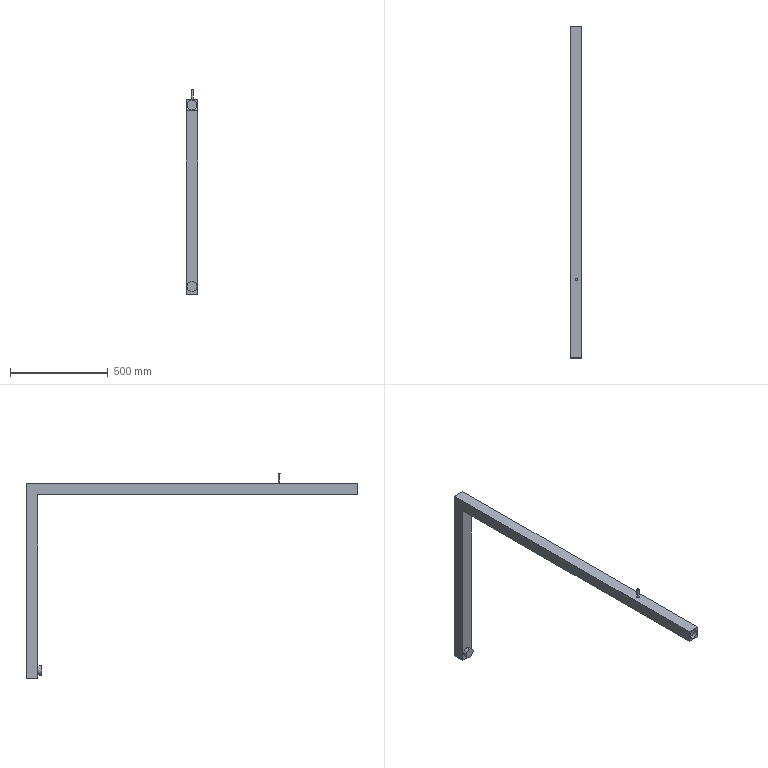Part | SolidWorks | features BaseBody 1 | 1 solid | 17 faces | box 60 x 1700 x 1049 mm | volume 9509525 mm3 | plane 11 | cylinder 6 | commonest cylinder face diameters 50 x4 12 x2
STEP:
#1=CARTESIAN_POINT('',(0.,1699.2,-991.929));
#2=VERTEX_POINT('',#1);
#3=CARTESIAN_POINT('',(0.,1699.2,-1041.929));
#4=VERTEX_POINT('',#3);
#5=CARTESIAN_POINT('',(0.,1699.2,-1016.929));
#6=DIRECTION('',(0.,1.,0.));
#7=DIRECTION('',(0.,0.,1.));
#8=AXIS2_PLACEMENT_3D('',#5,#6,#7);
#9=CIRCLE('',#8,25.);
#10=EDGE_CURVE('',#2,#4,#9,.T.);
#11=ORIENTED_EDGE('',*,*,#10,.T.);
#12=CARTESIAN_POINT('',(0.,1719.2,-1041.929));
#13=VERTEX_POINT('',#12);
#14=CARTESIAN_POINT('',(0.,1699.2,-1041.929));
#15=DIRECTION('',(0.,1.,0.));
#16=VECTOR('',#15,1000.);
#17=LINE('',#14,#16);
#18=EDGE_CURVE('',#4,#13,#17,.T.);
#19=ORIENTED_EDGE('',*,*,#18,.T.);
#20=CARTESIAN_POINT('',(0.,1719.2,-991.929));
#21=VERTEX_POINT('',#20);
#22=CARTESIAN_POINT('',(0.,1719.2,-1016.929));
#23=DIRECTION('',(0.,-1.,0.));
#24=DIRECTION('',(0.,0.,1.));
#25=AXIS2_PLACEMENT_3D('',#22,#23,#24);
#26=CIRCLE('',#25,25.);
#27=EDGE_CURVE('',#13,#21,#26,.T.);
#28=ORIENTED_EDGE('',*,*,#27,.T.);
#29=CARTESIAN_POINT('',(0.,1699.2,-991.929));
#30=DIRECTION('',(0.,1.,0.));
#31=VECTOR('',#30,1000.);
#32=LINE('',#29,#31);
#33=EDGE_CURVE('',#2,#21,#32,.T.);
#34=ORIENTED_EDGE('',*,*,#33,.F.);
#35=EDGE_LOOP('',(#11,#19,#28,#34));
#36=FACE_OUTER_BOUND('',#35,.T.);
#37=CARTESIAN_POINT('',(0.,1699.2,-1016.929));
#38=DIRECTION('',(0.,1.,0.));
#39=DIRECTION('',(0.,0.,1.));
#40=AXIS2_PLACEMENT_3D('',#37,#38,#39);
#41=CYLINDRICAL_SURFACE('',#40,25.);
#42=ADVANCED_FACE('',(#36),#41,.T.);
#43=CARTESIAN_POINT('',(0.,99.2,-62.879));
#44=VERTEX_POINT('',#43);
#45=CARTESIAN_POINT('',(0.,99.2,-112.879));
#46=VERTEX_POINT('',#45);
#47=CARTESIAN_POINT('',(0.,99.2,-87.879));
#48=DIRECTION('',(0.,-1.,0.));
#49=DIRECTION('',(0.,0.,-1.));
#50=AXIS2_PLACEMENT_3D('',#47,#48,#49);
#51=CIRCLE('',#50,25.);
#52=EDGE_CURVE('',#44,#46,#51,.T.);
#53=ORIENTED_EDGE('',*,*,#52,.F.);
#54=CARTESIAN_POINT('',(0.,79.2,-62.879));
#55=VERTEX_POINT('',#54);
#56=CARTESIAN_POINT('',(0.,99.2,-62.879));
#57=DIRECTION('',(0.,-1.,0.));
#58=VECTOR('',#57,1000.);
#59=LINE('',#56,#58);
#60=EDGE_CURVE('',#44,#55,#59,.T.);
#61=ORIENTED_EDGE('',*,*,#60,.T.);
#62=CARTESIAN_POINT('',(0.,79.2,-112.879));
#63=VERTEX_POINT('',#62);
#64=CARTESIAN_POINT('',(0.,79.2,-87.879));
#65=DIRECTION('',(0.,-1.,0.));
#66=DIRECTION('',(0.,0.,-1.));
#67=AXIS2_PLACEMENT_3D('',#64,#65,#66);
#68=CIRCLE('',#67,25.);
#69=EDGE_CURVE('',#55,#63,#68,.T.);
#70=ORIENTED_EDGE('',*,*,#69,.T.);
#71=CARTESIAN_POINT('',(0.,99.2,-112.879));
#72=DIRECTION('',(0.,-1.,0.));
#73=VECTOR('',#72,1000.);
#74=LINE('',#71,#73);
#75=EDGE_CURVE('',#46,#63,#74,.T.);
#76=ORIENTED_EDGE('',*,*,#75,.F.);
#77=EDGE_LOOP('',(#53,#61,#70,#76));
#78=FACE_OUTER_BOUND('',#77,.T.);
#79=CARTESIAN_POINT('',(0.,99.2,-87.879));
#80=DIRECTION('',(0.,-1.,0.));
#81=DIRECTION('',(0.,0.,-1.));
#82=AXIS2_PLACEMENT_3D('',#79,#80,#81);
#83=CYLINDRICAL_SURFACE('',#82,25.);
#84=ADVANCED_FACE('',(#78),#83,.F.);
#85=CARTESIAN_POINT('',(-4.497,482.123,-9.029));
#86=VERTEX_POINT('',#85);
#87=CARTESIAN_POINT('',(7.503,482.123,-9.029));
#88=VERTEX_POINT('',#87);
#89=CARTESIAN_POINT('',(1.503,482.123,-9.029));
#90=DIRECTION('',(0.,0.,-1.));
#91=DIRECTION('',(-1.,0.,0.));
#92=AXIS2_PLACEMENT_3D('',#89,#90,#91);
#93=CIRCLE('',#92,6.);
#94=EDGE_CURVE('',#86,#88,#93,.T.);
#95=ORIENTED_EDGE('',*,*,#94,.T.);
#96=CARTESIAN_POINT('',(7.503,482.123,-57.879));
#97=VERTEX_POINT('',#96);
#98=CARTESIAN_POINT('',(7.503,482.123,7.942));
#99=DIRECTION('',(0.,0.,-1.));
#100=VECTOR('',#99,1000.);
#101=LINE('',#98,#100);
#102=EDGE_CURVE('',#88,#97,#101,.T.);
#103=ORIENTED_EDGE('',*,*,#102,.T.);
#104=CARTESIAN_POINT('',(-4.497,482.123,-57.879));
#105=VERTEX_POINT('',#104);
#106=CARTESIAN_POINT('',(1.503,482.123,-57.879));
#107=DIRECTION('',(0.,0.,1.));
#108=DIRECTION('',(-1.,0.,0.));
#109=AXIS2_PLACEMENT_3D('',#106,#107,#108);
#110=CIRCLE('',#109,6.);
#111=EDGE_CURVE('',#97,#105,#110,.T.);
#112=ORIENTED_EDGE('',*,*,#111,.T.);
#113=CARTESIAN_POINT('',(-4.497,482.123,7.942));
#114=DIRECTION('',(0.,0.,-1.));
#115=VECTOR('',#114,1000.);
#116=LINE('',#113,#115);
#117=EDGE_CURVE('',#86,#105,#116,.T.);
#118=ORIENTED_EDGE('',*,*,#117,.F.);
#119=EDGE_LOOP('',(#95,#103,#112,#118));
#120=FACE_OUTER_BOUND('',#119,.T.);
#121=CARTESIAN_POINT('',(1.503,482.123,7.942));
#122=DIRECTION('',(0.,0.,-1.));
#123=DIRECTION('',(-1.,0.,0.));
#124=AXIS2_PLACEMENT_3D('',#121,#122,#123);
#125=CYLINDRICAL_SURFACE('',#124,6.);
#126=ADVANCED_FACE('',(#120),#125,.T.);
#127=CARTESIAN_POINT('',(30.,1719.2,-1057.879));
#128=VERTEX_POINT('',#127);
#129=CARTESIAN_POINT('',(30.,1779.2,-1057.879));
#130=VERTEX_POINT('',#129);
#131=CARTESIAN_POINT('',(30.,1133.527,-1057.879));
#132=DIRECTION('',(0.,1.,0.));
#133=VECTOR('',#132,1000.);
#134=LINE('',#131,#133);
#135=EDGE_CURVE('',#128,#130,#134,.T.);
#136=ORIENTED_EDGE('',*,*,#135,.T.);
#137=CARTESIAN_POINT('',(30.,1779.2,-57.879));
#138=VERTEX_POINT('',#137);
#139=CARTESIAN_POINT('',(30.,1779.2,-57.879));
#140=DIRECTION('',(0.,0.,1.));
#141=VECTOR('',#140,1000.);
#142=LINE('',#139,#141);
#143=EDGE_CURVE('',#130,#138,#142,.T.);
#144=ORIENTED_EDGE('',*,*,#143,.T.);
#145=CARTESIAN_POINT('',(30.,79.2,-57.879));
#146=VERTEX_POINT('',#145);
#147=CARTESIAN_POINT('',(30.,1133.527,-57.879));
#148=DIRECTION('',(0.,-1.,0.));
#149=VECTOR('',#148,1000.);
#150=LINE('',#147,#149);
#151=EDGE_CURVE('',#138,#146,#150,.T.);
#152=ORIENTED_EDGE('',*,*,#151,.T.);
#153=CARTESIAN_POINT('',(30.,79.2,-117.879));
#154=VERTEX_POINT('',#153);
#155=CARTESIAN_POINT('',(30.,79.2,-57.879));
#156=DIRECTION('',(0.,0.,-1.));
#157=VECTOR('',#156,1000.);
#158=LINE('',#155,#157);
#159=EDGE_CURVE('',#146,#154,#158,.T.);
#160=ORIENTED_EDGE('',*,*,#159,.T.);
#161=CARTESIAN_POINT('',(30.,1719.2,-117.879));
#162=VERTEX_POINT('',#161);
#163=CARTESIAN_POINT('',(30.,1133.527,-117.879));
#164=DIRECTION('',(0.,1.,0.));
#165=VECTOR('',#164,1000.);
#166=LINE('',#163,#165);
#167=EDGE_CURVE('',#154,#162,#166,.T.);
#168=ORIENTED_EDGE('',*,*,#167,.T.);
#169=CARTESIAN_POINT('',(30.,1719.2,-57.879));
#170=DIRECTION('',(0.,0.,-1.));
#171=VECTOR('',#170,1000.);
#172=LINE('',#169,#171);
#173=EDGE_CURVE('',#162,#128,#172,.T.);
#174=ORIENTED_EDGE('',*,*,#173,.T.);
#175=EDGE_LOOP('',(#136,#144,#152,#160,#168,#174));
#176=FACE_OUTER_BOUND('',#175,.T.);
#177=CARTESIAN_POINT('',(30.,1133.527,-57.879));
#178=DIRECTION('',(1.,0.,0.));
#179=DIRECTION('',(0.,0.,-1.));
#180=AXIS2_PLACEMENT_3D('',#177,#178,#179);
#181=PLANE('',#180);
#182=ADVANCED_FACE('',(#176),#181,.T.);
#183=CARTESIAN_POINT('',(-30.,1779.2,-57.879));
#184=VERTEX_POINT('',#183);
#185=CARTESIAN_POINT('',(30.,1779.2,-57.879));
#186=DIRECTION('',(-1.,0.,0.));
#187=VECTOR('',#186,1000.);
#188=LINE('',#185,#187);
#189=EDGE_CURVE('',#138,#184,#188,.T.);
#190=ORIENTED_EDGE('',*,*,#189,.F.);
#191=ORIENTED_EDGE('',*,*,#143,.F.);
#192=CARTESIAN_POINT('',(-30.,1779.2,-1057.879));
#193=VERTEX_POINT('',#192);
#194=CARTESIAN_POINT('',(30.,1779.2,-1057.879));
#195=DIRECTION('',(1.,0.,0.));
#196=VECTOR('',#195,1000.);
#197=LINE('',#194,#196);
#198=EDGE_CURVE('',#193,#130,#197,.T.);
#199=ORIENTED_EDGE('',*,*,#198,.F.);
#200=CARTESIAN_POINT('',(-30.,1779.2,-57.879));
#201=DIRECTION('',(0.,0.,-1.));
#202=VECTOR('',#201,1000.);
#203=LINE('',#200,#202);
#204=EDGE_CURVE('',#184,#193,#203,.T.);
#205=ORIENTED_EDGE('',*,*,#204,.F.);
#206=EDGE_LOOP('',(#190,#191,#199,#205));
#207=FACE_OUTER_BOUND('',#206,.T.);
#208=CARTESIAN_POINT('',(30.,1779.2,-57.879));
#209=DIRECTION('',(0.,-1.,0.));
#210=DIRECTION('',(0.,0.,-1.));
#211=AXIS2_PLACEMENT_3D('',#208,#209,#210);
#212=PLANE('',#211);
#213=ADVANCED_FACE('',(#207),#212,.F.);
#214=ORIENTED_EDGE('',*,*,#198,.T.);
#215=ORIENTED_EDGE('',*,*,#135,.F.);
#216=CARTESIAN_POINT('',(-30.,1719.2,-1057.879));
#217=VERTEX_POINT('',#216);
#218=CARTESIAN_POINT('',(30.,1719.2,-1057.879));
#219=DIRECTION('',(1.,0.,0.));
#220=VECTOR('',#219,1000.);
#221=LINE('',#218,#220);
#222=EDGE_CURVE('',#217,#128,#221,.T.);
#223=ORIENTED_EDGE('',*,*,#222,.F.);
#224=CARTESIAN_POINT('',(-30.,1779.2,-1057.879));
#225=DIRECTION('',(0.,-1.,0.));
#226=VECTOR('',#225,1000.);
#227=LINE('',#224,#226);
#228=EDGE_CURVE('',#193,#217,#227,.T.);
#229=ORIENTED_EDGE('',*,*,#228,.F.);
#230=EDGE_LOOP('',(#214,#215,#223,#229));
#231=FACE_OUTER_BOUND('',#230,.T.);
#232=CARTESIAN_POINT('',(30.,1779.2,-1057.879));
#233=DIRECTION('',(0.,0.,1.));
#234=DIRECTION('',(1.,0.,0.));
#235=AXIS2_PLACEMENT_3D('',#232,#233,#234);
#236=PLANE('',#235);
#237=ADVANCED_FACE('',(#231),#236,.F.);
#238=CARTESIAN_POINT('',(0.,1719.2,-1016.929));
#239=DIRECTION('',(0.,-1.,0.));
#240=DIRECTION('',(0.,0.,1.));
#241=AXIS2_PLACEMENT_3D('',#238,#239,#240);
#242=CIRCLE('',#241,25.);
#243=EDGE_CURVE('',#21,#13,#242,.T.);
#244=ORIENTED_EDGE('',*,*,#243,.F.);
#245=ORIENTED_EDGE('',*,*,#27,.F.);
#246=EDGE_LOOP('',(#244,#245));
#247=FACE_BOUND('',#246,.T.);
#248=ORIENTED_EDGE('',*,*,#222,.T.);
#249=ORIENTED_EDGE('',*,*,#173,.F.);
#250=CARTESIAN_POINT('',(-30.,1719.2,-117.879));
#251=VERTEX_POINT('',#250);
#252=CARTESIAN_POINT('',(30.,1719.2,-117.879));
#253=DIRECTION('',(1.,0.,0.));
#254=VECTOR('',#253,1000.);
#255=LINE('',#252,#254);
#256=EDGE_CURVE('',#251,#162,#255,.T.);
#257=ORIENTED_EDGE('',*,*,#256,.F.);
#258=CARTESIAN_POINT('',(-30.,1719.2,-117.879));
#259=DIRECTION('',(0.,0.,1.));
#260=VECTOR('',#259,1000.);
#261=LINE('',#258,#260);
#262=EDGE_CURVE('',#217,#251,#261,.T.);
#263=ORIENTED_EDGE('',*,*,#262,.F.);
#264=EDGE_LOOP('',(#248,#249,#257,#263));
#265=FACE_OUTER_BOUND('',#264,.T.);
#266=CARTESIAN_POINT('',(30.,1719.2,-117.879));
#267=DIRECTION('',(0.,1.,0.));
#268=DIRECTION('',(0.,0.,1.));
#269=AXIS2_PLACEMENT_3D('',#266,#267,#268);
#270=PLANE('',#269);
#271=ADVANCED_FACE('',(#247,#265),#270,.F.);
#272=ORIENTED_EDGE('',*,*,#256,.T.);
#273=ORIENTED_EDGE('',*,*,#167,.F.);
#274=CARTESIAN_POINT('',(-30.,79.2,-117.879));
#275=VERTEX_POINT('',#274);
#276=CARTESIAN_POINT('',(30.,79.2,-117.879));
#277=DIRECTION('',(1.,0.,0.));
#278=VECTOR('',#277,1000.);
#279=LINE('',#276,#278);
#280=EDGE_CURVE('',#275,#154,#279,.T.);
#281=ORIENTED_EDGE('',*,*,#280,.F.);
#282=CARTESIAN_POINT('',(-30.,1719.2,-117.879));
#283=DIRECTION('',(0.,-1.,0.));
#284=VECTOR('',#283,1000.);
#285=LINE('',#282,#284);
#286=EDGE_CURVE('',#251,#275,#285,.T.);
#287=ORIENTED_EDGE('',*,*,#286,.F.);
#288=EDGE_LOOP('',(#272,#273,#281,#287));
#289=FACE_OUTER_BOUND('',#288,.T.);
#290=CARTESIAN_POINT('',(30.,1719.2,-117.879));
#291=DIRECTION('',(0.,0.,1.));
#292=DIRECTION('',(1.,0.,0.));
#293=AXIS2_PLACEMENT_3D('',#290,#291,#292);
#294=PLANE('',#293);
#295=ADVANCED_FACE('',(#289),#294,.F.);
#296=ORIENTED_EDGE('',*,*,#280,.T.);
#297=ORIENTED_EDGE('',*,*,#159,.F.);
#298=CARTESIAN_POINT('',(-30.,79.2,-57.879));
#299=VERTEX_POINT('',#298);
#300=CARTESIAN_POINT('',(30.,79.2,-57.879));
#301=DIRECTION('',(1.,0.,0.));
#302=VECTOR('',#301,1000.);
#303=LINE('',#300,#302);
#304=EDGE_CURVE('',#299,#146,#303,.T.);
#305=ORIENTED_EDGE('',*,*,#304,.F.);
#306=CARTESIAN_POINT('',(-30.,79.2,-57.879));
#307=DIRECTION('',(0.,0.,1.));
#308=VECTOR('',#307,1000.);
#309=LINE('',#306,#308);
#310=EDGE_CURVE('',#275,#299,#309,.T.);
#311=ORIENTED_EDGE('',*,*,#310,.F.);
#312=EDGE_LOOP('',(#296,#297,#305,#311));
#313=FACE_OUTER_BOUND('',#312,.T.);
#314=CARTESIAN_POINT('',(0.,79.2,-87.879));
#315=DIRECTION('',(0.,-1.,0.));
#316=DIRECTION('',(0.,0.,-1.));
#317=AXIS2_PLACEMENT_3D('',#314,#315,#316);
#318=CIRCLE('',#317,25.);
#319=EDGE_CURVE('',#63,#55,#318,.T.);
#320=ORIENTED_EDGE('',*,*,#319,.F.);
#321=ORIENTED_EDGE('',*,*,#69,.F.);
#322=EDGE_LOOP('',(#320,#321));
#323=FACE_BOUND('',#322,.T.);
#324=CARTESIAN_POINT('',(30.,79.2,-57.879));
#325=DIRECTION('',(0.,1.,0.));
#326=DIRECTION('',(0.,0.,1.));
#327=AXIS2_PLACEMENT_3D('',#324,#325,#326);
#328=PLANE('',#327);
#329=ADVANCED_FACE('',(#313,#323),#328,.F.);
#330=CARTESIAN_POINT('',(1.503,482.123,-57.879));
#331=DIRECTION('',(0.,0.,1.));
#332=DIRECTION('',(-1.,0.,0.));
#333=AXIS2_PLACEMENT_3D('',#330,#331,#332);
#334=CIRCLE('',#333,6.);
#335=EDGE_CURVE('',#105,#97,#334,.T.);
#336=ORIENTED_EDGE('',*,*,#335,.F.);
#337=ORIENTED_EDGE('',*,*,#111,.F.);
#338=EDGE_LOOP('',(#336,#337));
#339=FACE_BOUND('',#338,.T.);
#340=ORIENTED_EDGE('',*,*,#304,.T.);
#341=ORIENTED_EDGE('',*,*,#151,.F.);
#342=ORIENTED_EDGE('',*,*,#189,.T.);
#343=CARTESIAN_POINT('',(-30.,1644.344,-57.879));
#344=DIRECTION('',(0.,1.,0.));
#345=VECTOR('',#344,1000.);
#346=LINE('',#343,#345);
#347=EDGE_CURVE('',#299,#184,#346,.T.);
#348=ORIENTED_EDGE('',*,*,#347,.F.);
#349=EDGE_LOOP('',(#340,#341,#342,#348));
#350=FACE_OUTER_BOUND('',#349,.T.);
#351=CARTESIAN_POINT('',(30.,1644.344,-57.879));
#352=DIRECTION('',(0.,0.,-1.));
#353=DIRECTION('',(-1.,0.,0.));
#354=AXIS2_PLACEMENT_3D('',#351,#352,#353);
#355=PLANE('',#354);
#356=ADVANCED_FACE('',(#339,#350),#355,.F.);
#357=ORIENTED_EDGE('',*,*,#204,.T.);
#358=ORIENTED_EDGE('',*,*,#228,.T.);
#359=ORIENTED_EDGE('',*,*,#262,.T.);
#360=ORIENTED_EDGE('',*,*,#286,.T.);
#361=ORIENTED_EDGE('',*,*,#310,.T.);
#362=ORIENTED_EDGE('',*,*,#347,.T.);
#363=EDGE_LOOP('',(#357,#358,#359,#360,#361,#362));
#364=FACE_OUTER_BOUND('',#363,.T.);
#365=CARTESIAN_POINT('',(-30.,1133.527,-57.879));
#366=DIRECTION('',(1.,0.,0.));
#367=DIRECTION('',(0.,0.,-1.));
#368=AXIS2_PLACEMENT_3D('',#365,#366,#367);
#369=PLANE('',#368);
#370=ADVANCED_FACE('',(#364),#369,.F.);
#371=ORIENTED_EDGE('',*,*,#18,.F.);
#372=CARTESIAN_POINT('',(0.,1699.2,-1016.929));
#373=DIRECTION('',(0.,1.,0.));
#374=DIRECTION('',(0.,0.,1.));
#375=AXIS2_PLACEMENT_3D('',#372,#373,#374);
#376=CIRCLE('',#375,25.);
#377=EDGE_CURVE('',#4,#2,#376,.T.);
#378=ORIENTED_EDGE('',*,*,#377,.T.);
#379=ORIENTED_EDGE('',*,*,#33,.T.);
#380=ORIENTED_EDGE('',*,*,#243,.T.);
#381=EDGE_LOOP('',(#371,#378,#379,#380));
#382=FACE_OUTER_BOUND('',#381,.T.);
#383=CARTESIAN_POINT('',(0.,1699.2,-1016.929));
#384=DIRECTION('',(0.,1.,0.));
#385=DIRECTION('',(0.,0.,1.));
#386=AXIS2_PLACEMENT_3D('',#383,#384,#385);
#387=CYLINDRICAL_SURFACE('',#386,25.);
#388=ADVANCED_FACE('',(#382),#387,.T.);
#389=ORIENTED_EDGE('',*,*,#60,.F.);
#390=CARTESIAN_POINT('',(0.,99.2,-87.879));
#391=DIRECTION('',(0.,-1.,0.));
#392=DIRECTION('',(0.,0.,-1.));
#393=AXIS2_PLACEMENT_3D('',#390,#391,#392);
#394=CIRCLE('',#393,25.);
#395=EDGE_CURVE('',#46,#44,#394,.T.);
#396=ORIENTED_EDGE('',*,*,#395,.F.);
#397=ORIENTED_EDGE('',*,*,#75,.T.);
#398=ORIENTED_EDGE('',*,*,#319,.T.);
#399=EDGE_LOOP('',(#389,#396,#397,#398));
#400=FACE_OUTER_BOUND('',#399,.T.);
#401=CARTESIAN_POINT('',(0.,99.2,-87.879));
#402=DIRECTION('',(0.,-1.,0.));
#403=DIRECTION('',(0.,0.,-1.));
#404=AXIS2_PLACEMENT_3D('',#401,#402,#403);
#405=CYLINDRICAL_SURFACE('',#404,25.);
#406=ADVANCED_FACE('',(#400),#405,.F.);
#407=ORIENTED_EDGE('',*,*,#102,.F.);
#408=CARTESIAN_POINT('',(1.503,482.123,-9.029));
#409=DIRECTION('',(0.,0.,-1.));
#410=DIRECTION('',(-1.,0.,0.));
#411=AXIS2_PLACEMENT_3D('',#408,#409,#410);
#412=CIRCLE('',#411,6.);
#413=EDGE_CURVE('',#88,#86,#412,.T.);
#414=ORIENTED_EDGE('',*,*,#413,.T.);
#415=ORIENTED_EDGE('',*,*,#117,.T.);
#416=ORIENTED_EDGE('',*,*,#335,.T.);
#417=EDGE_LOOP('',(#407,#414,#415,#416));
#418=FACE_OUTER_BOUND('',#417,.T.);
#419=CARTESIAN_POINT('',(1.503,482.123,7.942));
#420=DIRECTION('',(0.,0.,-1.));
#421=DIRECTION('',(-1.,0.,0.));
#422=AXIS2_PLACEMENT_3D('',#419,#420,#421);
#423=CYLINDRICAL_SURFACE('',#422,6.);
#424=ADVANCED_FACE('',(#418),#423,.T.);
#425=ORIENTED_EDGE('',*,*,#10,.F.);
#426=ORIENTED_EDGE('',*,*,#377,.F.);
#427=EDGE_LOOP('',(#425,#426));
#428=FACE_OUTER_BOUND('',#427,.T.);
#429=CARTESIAN_POINT('',(0.,1699.2,-1016.929));
#430=DIRECTION('',(0.,-1.,0.));
#431=DIRECTION('',(0.,0.,-1.));
#432=AXIS2_PLACEMENT_3D('',#429,#430,#431);
#433=PLANE('',#432);
#434=ADVANCED_FACE('',(#428),#433,.T.);
#435=ORIENTED_EDGE('',*,*,#395,.T.);
#436=ORIENTED_EDGE('',*,*,#52,.T.);
#437=EDGE_LOOP('',(#435,#436));
#438=FACE_OUTER_BOUND('',#437,.T.);
#439=CARTESIAN_POINT('',(0.,99.2,-87.879));
#440=DIRECTION('',(0.,-1.,0.));
#441=DIRECTION('',(0.,0.,-1.));
#442=AXIS2_PLACEMENT_3D('',#439,#440,#441);
#443=PLANE('',#442);
#444=ADVANCED_FACE('',(#438),#443,.T.);
#445=ORIENTED_EDGE('',*,*,#94,.F.);
#446=ORIENTED_EDGE('',*,*,#413,.F.);
#447=EDGE_LOOP('',(#445,#446));
#448=FACE_OUTER_BOUND('',#447,.T.);
#449=CARTESIAN_POINT('',(-3.256,465.802,-9.029));
#450=DIRECTION('',(0.,0.,1.));
#451=DIRECTION('',(1.,0.,0.));
#452=AXIS2_PLACEMENT_3D('',#449,#450,#451);
#453=PLANE('',#452);
#454=ADVANCED_FACE('',(#448),#453,.T.);
#455=CLOSED_SHELL('',(#42,#84,#126,#182,#213,#237,#271,#295,#329,#356,#370,#388,#406,#424,#434,#444,#454));
#456=MANIFOLD_SOLID_BREP('',#455);
#457=CARTESIAN_POINT('',(0.,0.,0.));
#458=DIRECTION('',(0.,0.,1.));
#459=DIRECTION('',(1.,0.,0.));
#460=AXIS2_PLACEMENT_3D('',#457,#458,#459);
#461=(LENGTH_UNIT()NAMED_UNIT(*)SI_UNIT(.MILLI.,.METRE.));
#462=UNCERTAINTY_MEASURE_WITH_UNIT(LENGTH_MEASURE(0.00001),#461,'','');
#463=(NAMED_UNIT(*)PLANE_ANGLE_UNIT()SI_UNIT($,.RADIAN.));
#464=(NAMED_UNIT(*)SI_UNIT($,.STERADIAN.)SOLID_ANGLE_UNIT());
#465=(GEOMETRIC_REPRESENTATION_CONTEXT(3)GLOBAL_UNCERTAINTY_ASSIGNED_CONTEXT((#462))GLOBAL_UNIT_ASSIGNED_CONTEXT((#461,#463,#464))REPRESENTATION_CONTEXT('',''));
#466=ADVANCED_BREP_SHAPE_REPRESENTATION('',(#456,#460),#465);